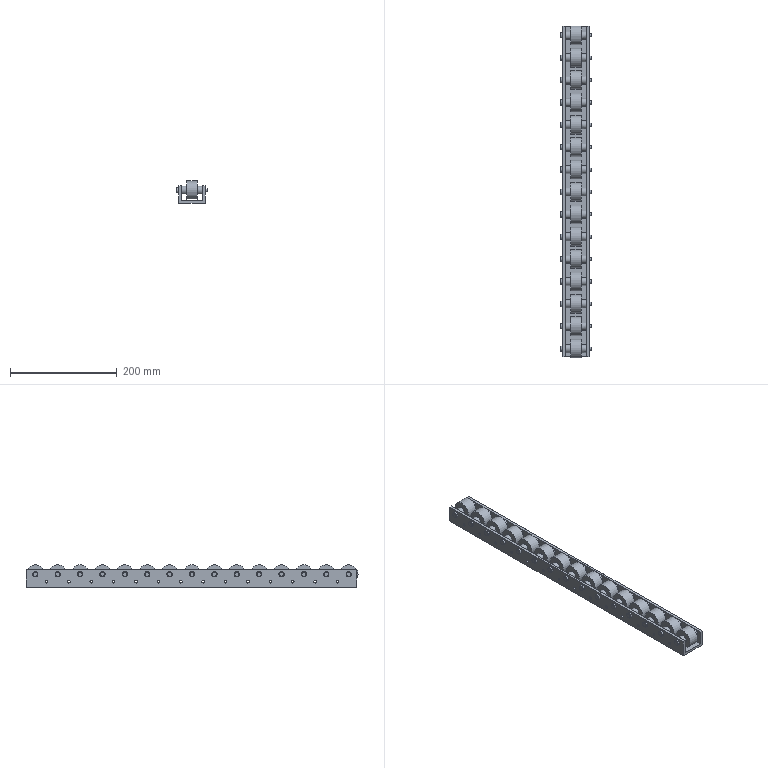Part | NX | features solid 2 | 1 solid | 188 faces | box 60 x 623 x 41.5 mm | volume 669090 mm3 | cylinder 103 | plane 69 | cone 15 | spline 1 | commonest cylinder face diameters 15 x30 5 x28 6 x15 10 x15 35 x15